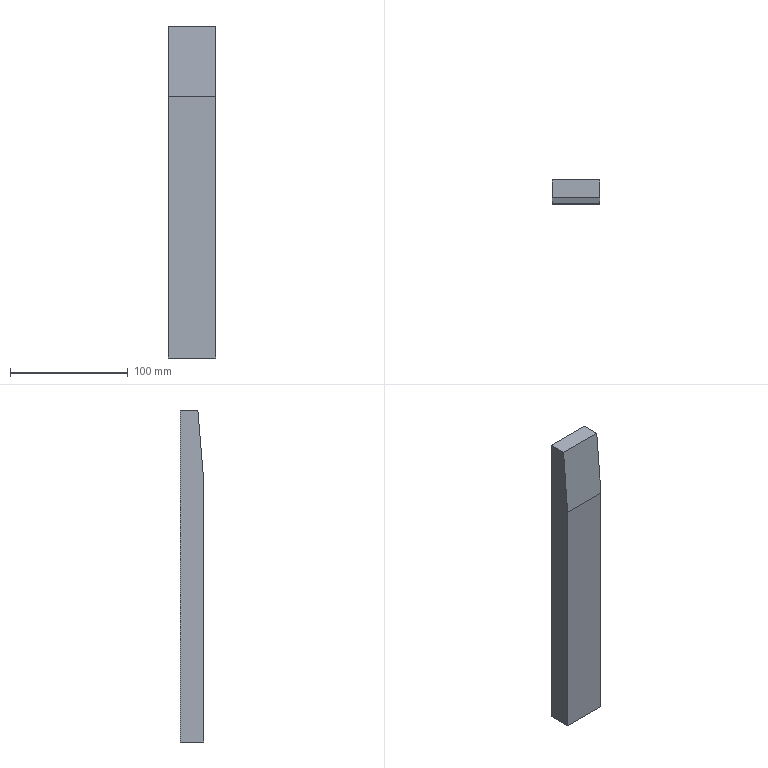Part | SolidWorks | features BaseBody 1 | 1 solid | 7 faces | box 40 x 20 x 282.5 mm | volume 220000 mm3 | plane 7
STEP:
#1=CARTESIAN_POINT('',(-147.496,1780.044,-23.5));
#2=VERTEX_POINT('',#1);
#3=CARTESIAN_POINT('',(-147.496,1780.044,-306.));
#4=VERTEX_POINT('',#3);
#5=CARTESIAN_POINT('',(-147.496,1780.044,-103.5));
#6=DIRECTION('',(0.,0.,-1.));
#7=VECTOR('',#6,1000.);
#8=LINE('',#5,#7);
#9=EDGE_CURVE('',#2,#4,#8,.T.);
#10=ORIENTED_EDGE('',*,*,#9,.F.);
#11=CARTESIAN_POINT('',(-107.496,1780.044,-23.5));
#12=VERTEX_POINT('',#11);
#13=CARTESIAN_POINT('',(-127.496,1780.044,-23.5));
#14=DIRECTION('',(-1.,0.,0.));
#15=VECTOR('',#14,1000.);
#16=LINE('',#13,#15);
#17=EDGE_CURVE('',#12,#2,#16,.T.);
#18=ORIENTED_EDGE('',*,*,#17,.F.);
#19=CARTESIAN_POINT('',(-107.496,1780.044,-306.));
#20=VERTEX_POINT('',#19);
#21=CARTESIAN_POINT('',(-107.496,1780.044,-103.5));
#22=DIRECTION('',(0.,0.,1.));
#23=VECTOR('',#22,1000.);
#24=LINE('',#21,#23);
#25=EDGE_CURVE('',#20,#12,#24,.T.);
#26=ORIENTED_EDGE('',*,*,#25,.F.);
#27=CARTESIAN_POINT('',(-127.496,1780.044,-306.));
#28=DIRECTION('',(1.,0.,0.));
#29=VECTOR('',#28,1000.);
#30=LINE('',#27,#29);
#31=EDGE_CURVE('',#4,#20,#30,.T.);
#32=ORIENTED_EDGE('',*,*,#31,.F.);
#33=EDGE_LOOP('',(#10,#18,#26,#32));
#34=FACE_OUTER_BOUND('',#33,.T.);
#35=CARTESIAN_POINT('',(-127.496,1780.044,-103.5));
#36=DIRECTION('',(0.,-1.,0.));
#37=DIRECTION('',(0.,0.,-1.));
#38=AXIS2_PLACEMENT_3D('',#35,#36,#37);
#39=PLANE('',#38);
#40=ADVANCED_FACE('',(#34),#39,.F.);
#41=CARTESIAN_POINT('',(-147.496,1760.044,-306.));
#42=VERTEX_POINT('',#41);
#43=CARTESIAN_POINT('',(-107.496,1760.044,-306.));
#44=VERTEX_POINT('',#43);
#45=CARTESIAN_POINT('',(-147.496,1760.044,-306.));
#46=DIRECTION('',(1.,0.,0.));
#47=VECTOR('',#46,1000.);
#48=LINE('',#45,#47);
#49=EDGE_CURVE('',#42,#44,#48,.T.);
#50=ORIENTED_EDGE('',*,*,#49,.F.);
#51=CARTESIAN_POINT('',(-147.496,1760.044,-306.));
#52=DIRECTION('',(0.,-1.,0.));
#53=VECTOR('',#52,1000.);
#54=LINE('',#51,#53);
#55=EDGE_CURVE('',#4,#42,#54,.T.);
#56=ORIENTED_EDGE('',*,*,#55,.F.);
#57=ORIENTED_EDGE('',*,*,#31,.T.);
#58=CARTESIAN_POINT('',(-107.496,1760.044,-306.));
#59=DIRECTION('',(0.,1.,0.));
#60=VECTOR('',#59,1000.);
#61=LINE('',#58,#60);
#62=EDGE_CURVE('',#44,#20,#61,.T.);
#63=ORIENTED_EDGE('',*,*,#62,.F.);
#64=EDGE_LOOP('',(#50,#56,#57,#63));
#65=FACE_OUTER_BOUND('',#64,.T.);
#66=CARTESIAN_POINT('',(-147.496,1760.044,-306.));
#67=DIRECTION('',(0.,0.,1.));
#68=DIRECTION('',(1.,0.,0.));
#69=AXIS2_PLACEMENT_3D('',#66,#67,#68);
#70=PLANE('',#69);
#71=ADVANCED_FACE('',(#65),#70,.F.);
#72=CARTESIAN_POINT('',(-147.496,1765.044,-23.5));
#73=VERTEX_POINT('',#72);
#74=CARTESIAN_POINT('',(-147.496,1760.044,-23.5));
#75=DIRECTION('',(0.,-1.,0.));
#76=VECTOR('',#75,1000.);
#77=LINE('',#74,#76);
#78=EDGE_CURVE('',#2,#73,#77,.T.);
#79=ORIENTED_EDGE('',*,*,#78,.F.);
#80=ORIENTED_EDGE('',*,*,#9,.T.);
#81=ORIENTED_EDGE('',*,*,#55,.T.);
#82=CARTESIAN_POINT('',(-147.496,1760.044,-83.5));
#83=VERTEX_POINT('',#82);
#84=CARTESIAN_POINT('',(-147.496,1760.044,196.5));
#85=DIRECTION('',(0.,0.,-1.));
#86=VECTOR('',#85,1000.);
#87=LINE('',#84,#86);
#88=EDGE_CURVE('',#83,#42,#87,.T.);
#89=ORIENTED_EDGE('',*,*,#88,.F.);
#90=CARTESIAN_POINT('',(-147.496,1765.044,-23.5));
#91=DIRECTION('',(0.,-0.08305,-0.9965));
#92=VECTOR('',#91,1000.);
#93=LINE('',#90,#92);
#94=EDGE_CURVE('',#73,#83,#93,.T.);
#95=ORIENTED_EDGE('',*,*,#94,.F.);
#96=EDGE_LOOP('',(#79,#80,#81,#89,#95));
#97=FACE_OUTER_BOUND('',#96,.T.);
#98=CARTESIAN_POINT('',(-147.496,1760.044,196.5));
#99=DIRECTION('',(1.,0.,0.));
#100=DIRECTION('',(0.,0.,-1.));
#101=AXIS2_PLACEMENT_3D('',#98,#99,#100);
#102=PLANE('',#101);
#103=ADVANCED_FACE('',(#97),#102,.F.);
#104=CARTESIAN_POINT('',(-107.496,1765.044,-23.5));
#105=VERTEX_POINT('',#104);
#106=CARTESIAN_POINT('',(-107.496,1760.044,-23.5));
#107=DIRECTION('',(0.,-1.,0.));
#108=VECTOR('',#107,1000.);
#109=LINE('',#106,#108);
#110=EDGE_CURVE('',#12,#105,#109,.T.);
#111=ORIENTED_EDGE('',*,*,#110,.F.);
#112=ORIENTED_EDGE('',*,*,#17,.T.);
#113=ORIENTED_EDGE('',*,*,#78,.T.);
#114=CARTESIAN_POINT('',(-147.496,1765.044,-23.5));
#115=DIRECTION('',(-1.,0.,0.));
#116=VECTOR('',#115,1000.);
#117=LINE('',#114,#116);
#118=EDGE_CURVE('',#105,#73,#117,.T.);
#119=ORIENTED_EDGE('',*,*,#118,.F.);
#120=EDGE_LOOP('',(#111,#112,#113,#119));
#121=FACE_OUTER_BOUND('',#120,.T.);
#122=CARTESIAN_POINT('',(-147.496,1760.044,-23.5));
#123=DIRECTION('',(0.,0.,-1.));
#124=DIRECTION('',(-1.,0.,0.));
#125=AXIS2_PLACEMENT_3D('',#122,#123,#124);
#126=PLANE('',#125);
#127=ADVANCED_FACE('',(#121),#126,.F.);
#128=CARTESIAN_POINT('',(-107.496,1760.044,-83.5));
#129=VERTEX_POINT('',#128);
#130=CARTESIAN_POINT('',(-107.496,1760.044,196.5));
#131=DIRECTION('',(0.,0.,1.));
#132=VECTOR('',#131,1000.);
#133=LINE('',#130,#132);
#134=EDGE_CURVE('',#44,#129,#133,.T.);
#135=ORIENTED_EDGE('',*,*,#134,.F.);
#136=ORIENTED_EDGE('',*,*,#62,.T.);
#137=ORIENTED_EDGE('',*,*,#25,.T.);
#138=ORIENTED_EDGE('',*,*,#110,.T.);
#139=CARTESIAN_POINT('',(-107.496,1760.044,-83.5));
#140=DIRECTION('',(0.,0.08305,0.9965));
#141=VECTOR('',#140,1000.);
#142=LINE('',#139,#141);
#143=EDGE_CURVE('',#129,#105,#142,.T.);
#144=ORIENTED_EDGE('',*,*,#143,.F.);
#145=EDGE_LOOP('',(#135,#136,#137,#138,#144));
#146=FACE_OUTER_BOUND('',#145,.T.);
#147=CARTESIAN_POINT('',(-107.496,1760.044,196.5));
#148=DIRECTION('',(-1.,0.,0.));
#149=DIRECTION('',(0.,0.,1.));
#150=AXIS2_PLACEMENT_3D('',#147,#148,#149);
#151=PLANE('',#150);
#152=ADVANCED_FACE('',(#146),#151,.F.);
#153=ORIENTED_EDGE('',*,*,#49,.T.);
#154=ORIENTED_EDGE('',*,*,#134,.T.);
#155=CARTESIAN_POINT('',(-127.496,1760.044,-83.5));
#156=DIRECTION('',(-1.,0.,0.));
#157=VECTOR('',#156,1000.);
#158=LINE('',#155,#157);
#159=EDGE_CURVE('',#129,#83,#158,.T.);
#160=ORIENTED_EDGE('',*,*,#159,.T.);
#161=ORIENTED_EDGE('',*,*,#88,.T.);
#162=EDGE_LOOP('',(#153,#154,#160,#161));
#163=FACE_OUTER_BOUND('',#162,.T.);
#164=CARTESIAN_POINT('',(-127.496,1760.044,-103.5));
#165=DIRECTION('',(0.,-1.,0.));
#166=DIRECTION('',(0.,0.,-1.));
#167=AXIS2_PLACEMENT_3D('',#164,#165,#166);
#168=PLANE('',#167);
#169=ADVANCED_FACE('',(#163),#168,.T.);
#170=ORIENTED_EDGE('',*,*,#159,.F.);
#171=ORIENTED_EDGE('',*,*,#143,.T.);
#172=ORIENTED_EDGE('',*,*,#118,.T.);
#173=ORIENTED_EDGE('',*,*,#94,.T.);
#174=EDGE_LOOP('',(#170,#171,#172,#173));
#175=FACE_OUTER_BOUND('',#174,.T.);
#176=CARTESIAN_POINT('',(-127.496,1760.044,-83.5));
#177=DIRECTION('',(0.,-0.9965,0.08305));
#178=DIRECTION('',(0.,-0.08305,-0.9965));
#179=AXIS2_PLACEMENT_3D('',#176,#177,#178);
#180=PLANE('',#179);
#181=ADVANCED_FACE('',(#175),#180,.T.);
#182=CLOSED_SHELL('',(#40,#71,#103,#127,#152,#169,#181));
#183=MANIFOLD_SOLID_BREP('',#182);
#184=CARTESIAN_POINT('',(0.,0.,0.));
#185=DIRECTION('',(0.,0.,1.));
#186=DIRECTION('',(1.,0.,0.));
#187=AXIS2_PLACEMENT_3D('',#184,#185,#186);
#188=(LENGTH_UNIT()NAMED_UNIT(*)SI_UNIT(.MILLI.,.METRE.));
#189=UNCERTAINTY_MEASURE_WITH_UNIT(LENGTH_MEASURE(0.00001),#188,'','');
#190=(NAMED_UNIT(*)PLANE_ANGLE_UNIT()SI_UNIT($,.RADIAN.));
#191=(NAMED_UNIT(*)SI_UNIT($,.STERADIAN.)SOLID_ANGLE_UNIT());
#192=(GEOMETRIC_REPRESENTATION_CONTEXT(3)GLOBAL_UNCERTAINTY_ASSIGNED_CONTEXT((#189))GLOBAL_UNIT_ASSIGNED_CONTEXT((#188,#190,#191))REPRESENTATION_CONTEXT('',''));
#193=ADVANCED_BREP_SHAPE_REPRESENTATION('',(#183,#187),#192);